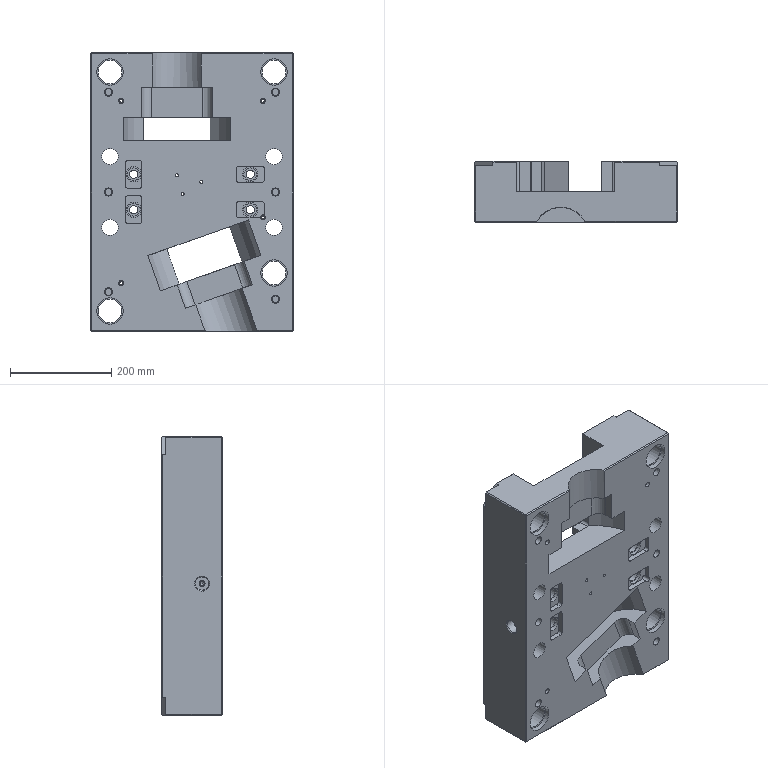Part | STEP file | B-PLATE_id558_x_t | 1 solid | 322 faces | box 400 x 120 x 550 mm | volume 16282853 mm3 | plane 203 | cylinder 107 | cone 12 | commonest cylinder face diameters 10 x45 16 x14 5.5 x4 8 x4 15.681 x4 25 x4